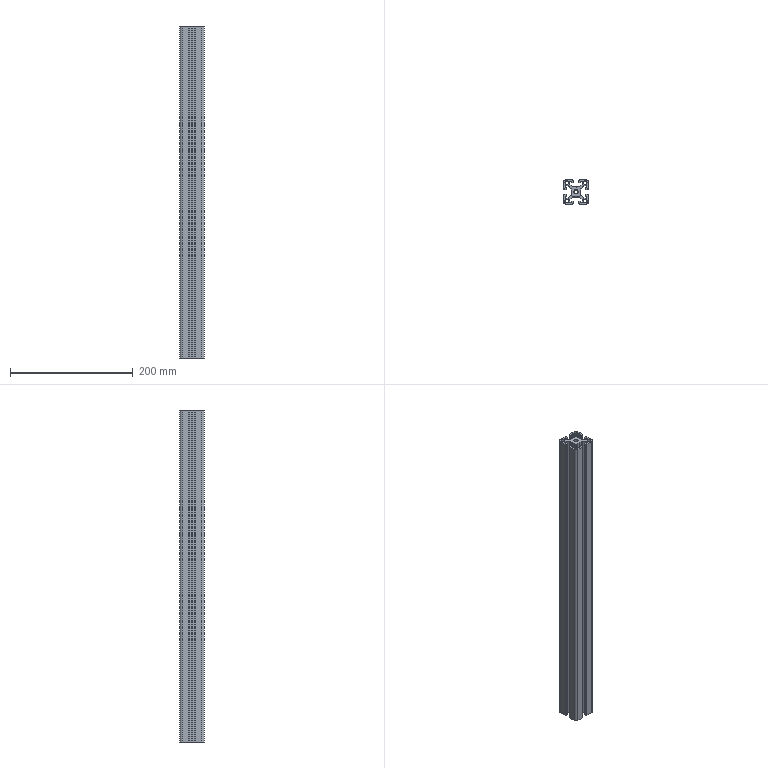Part | STEP file | HM-8-4040D-L540 | 1 solid | 176 faces | box 40 x 40 x 540 mm | volume 369715 mm3 | plane 90 | cylinder 86 | commonest cylinder face diameters 1 x40 0.4 x24 4 x8 6 x8 9 x4 6.8 x2